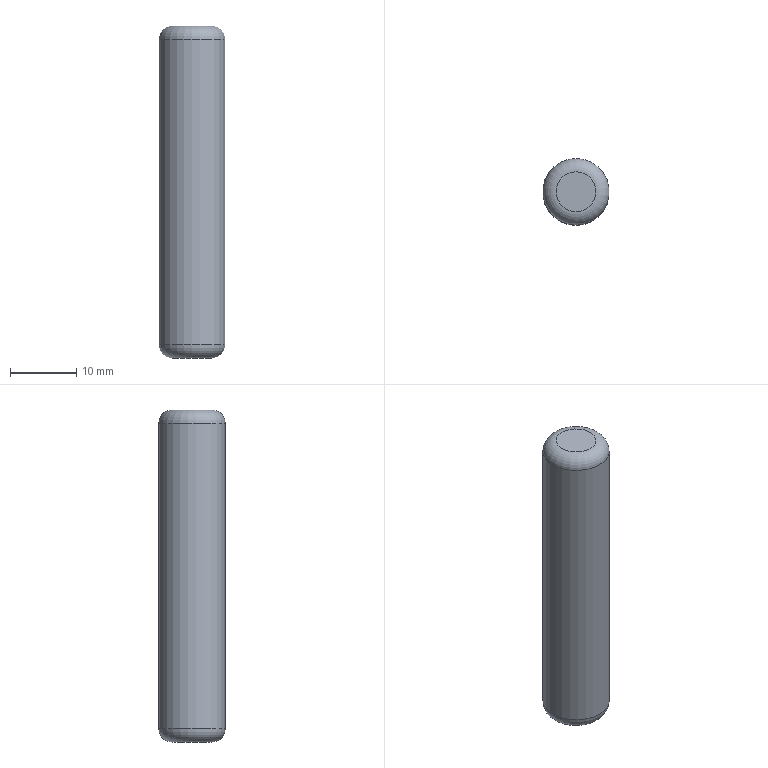Part | STEP file | D10-50_id1522_x_t | 1 solid | 5 faces | box 10 x 10 x 50 mm | volume 3878 mm3 | plane 2 | torus 2 | cylinder 1 | commonest cylinder face diameters 10 x1
STEP:
#1=CARTESIAN_POINT('',(-160.,247.,-22.));
#2=VERTEX_POINT('',#1);
#3=CARTESIAN_POINT('',(-160.,250.,-22.));
#4=DIRECTION('',(0.,0.,-1.));
#5=DIRECTION('',(0.,-1.,0.));
#6=AXIS2_PLACEMENT_3D('',#3,#4,#5);
#7=CIRCLE('',#6,3.);
#8=EDGE_CURVE('',#2,#2,#7,.T.);
#9=ORIENTED_EDGE('',*,*,#8,.F.);
#10=EDGE_LOOP('',(#9));
#11=FACE_OUTER_BOUND('',#10,.T.);
#12=CARTESIAN_POINT('',(-160.,250.,-22.));
#13=DIRECTION('',(0.,0.,1.));
#14=DIRECTION('',(0.,-1.,0.));
#15=AXIS2_PLACEMENT_3D('',#12,#13,#14);
#16=PLANE('',#15);
#17=ADVANCED_FACE('',(#11),#16,.T.);
#18=CARTESIAN_POINT('',(-160.,255.,-70.));
#19=VERTEX_POINT('',#18);
#20=CARTESIAN_POINT('',(-160.,250.,-70.));
#21=DIRECTION('',(0.,0.,-1.));
#22=DIRECTION('',(0.,1.,0.));
#23=AXIS2_PLACEMENT_3D('',#20,#21,#22);
#24=CIRCLE('',#23,5.);
#25=EDGE_CURVE('',#19,#19,#24,.T.);
#26=ORIENTED_EDGE('',*,*,#25,.F.);
#27=EDGE_LOOP('',(#26));
#28=FACE_BOUND('',#27,.T.);
#29=CARTESIAN_POINT('',(-160.,245.,-24.));
#30=VERTEX_POINT('',#29);
#31=CARTESIAN_POINT('',(-160.,250.,-24.));
#32=DIRECTION('',(0.,0.,1.));
#33=DIRECTION('',(0.,-1.,0.));
#34=AXIS2_PLACEMENT_3D('',#31,#32,#33);
#35=CIRCLE('',#34,5.);
#36=EDGE_CURVE('',#30,#30,#35,.T.);
#37=ORIENTED_EDGE('',*,*,#36,.F.);
#38=EDGE_LOOP('',(#37));
#39=FACE_BOUND('',#38,.T.);
#40=CARTESIAN_POINT('',(-160.,250.,-47.));
#41=DIRECTION('',(0.,0.,1.));
#42=DIRECTION('',(0.,-1.,0.));
#43=AXIS2_PLACEMENT_3D('',#40,#41,#42);
#44=CYLINDRICAL_SURFACE('',#43,5.);
#45=ADVANCED_FACE('',(#28,#39),#44,.T.);
#46=CARTESIAN_POINT('',(-160.,253.,-72.));
#47=VERTEX_POINT('',#46);
#48=CARTESIAN_POINT('',(-160.,250.,-72.));
#49=DIRECTION('',(0.,0.,1.));
#50=DIRECTION('',(0.,1.,0.));
#51=AXIS2_PLACEMENT_3D('',#48,#49,#50);
#52=CIRCLE('',#51,3.);
#53=EDGE_CURVE('',#47,#47,#52,.T.);
#54=ORIENTED_EDGE('',*,*,#53,.F.);
#55=EDGE_LOOP('',(#54));
#56=FACE_OUTER_BOUND('',#55,.T.);
#57=CARTESIAN_POINT('',(-160.,250.,-72.));
#58=DIRECTION('',(0.,0.,-1.));
#59=DIRECTION('',(0.,1.,0.));
#60=AXIS2_PLACEMENT_3D('',#57,#58,#59);
#61=PLANE('',#60);
#62=ADVANCED_FACE('',(#56),#61,.T.);
#63=ORIENTED_EDGE('',*,*,#8,.T.);
#64=EDGE_LOOP('',(#63));
#65=FACE_BOUND('',#64,.T.);
#66=ORIENTED_EDGE('',*,*,#36,.T.);
#67=EDGE_LOOP('',(#66));
#68=FACE_BOUND('',#67,.T.);
#69=CARTESIAN_POINT('',(-160.,250.,-24.));
#70=DIRECTION('',(0.,0.,1.));
#71=DIRECTION('',(0.,-1.,0.));
#72=AXIS2_PLACEMENT_3D('',#69,#70,#71);
#73=TOROIDAL_SURFACE('',#72,3.,2.);
#74=ADVANCED_FACE('',(#65,#68),#73,.T.);
#75=ORIENTED_EDGE('',*,*,#53,.T.);
#76=EDGE_LOOP('',(#75));
#77=FACE_BOUND('',#76,.T.);
#78=ORIENTED_EDGE('',*,*,#25,.T.);
#79=EDGE_LOOP('',(#78));
#80=FACE_BOUND('',#79,.T.);
#81=CARTESIAN_POINT('',(-160.,250.,-70.));
#82=DIRECTION('',(0.,0.,-1.));
#83=DIRECTION('',(0.,1.,0.));
#84=AXIS2_PLACEMENT_3D('',#81,#82,#83);
#85=TOROIDAL_SURFACE('',#84,3.,2.);
#86=ADVANCED_FACE('',(#77,#80),#85,.T.);
#87=CLOSED_SHELL('',(#17,#45,#62,#74,#86));
#88=MANIFOLD_SOLID_BREP('',#87);
#89=(LENGTH_UNIT()NAMED_UNIT(*)SI_UNIT(.MILLI.,.METRE.));
#90=UNCERTAINTY_MEASURE_WITH_UNIT(LENGTH_MEASURE(0.00002),#89,'','');
#91=(NAMED_UNIT(*)PLANE_ANGLE_UNIT()SI_UNIT($,.RADIAN.));
#92=PLANE_ANGLE_MEASURE_WITH_UNIT(PLANE_ANGLE_MEASURE(0.01745),#91);
#93=DIMENSIONAL_EXPONENTS(0.,0.,0.,0.,0.,0.,0.);
#94=(CONVERSION_BASED_UNIT('DEGREE',#92)NAMED_UNIT(#93)PLANE_ANGLE_UNIT());
#95=(NAMED_UNIT(*)SI_UNIT($,.STERADIAN.)SOLID_ANGLE_UNIT());
#96=(GEOMETRIC_REPRESENTATION_CONTEXT(3)GLOBAL_UNCERTAINTY_ASSIGNED_CONTEXT((#90))GLOBAL_UNIT_ASSIGNED_CONTEXT((#89,#94,#95))REPRESENTATION_CONTEXT('',''));
#97=ADVANCED_BREP_SHAPE_REPRESENTATION('',(#88),#96);